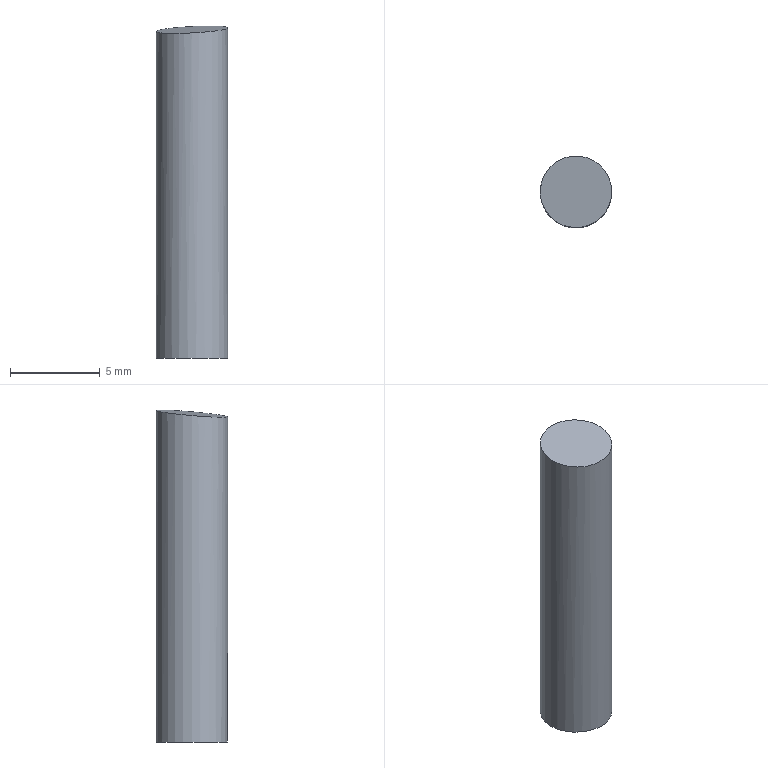Part | NX | features solid 2 | 1 solid | 3 faces | box 4 x 4 x 18.548 mm | volume 230.472 mm3 | plane 2 | cylinder 1 | commonest cylinder face diameters 4 x1
STEP:
#1=CARTESIAN_POINT('',(-212.753,0.1299,-24.));
#2=VERTEX_POINT('',#1);
#3=CARTESIAN_POINT('',(-210.753,0.1299,-24.));
#4=DIRECTION('',(0.,0.,-1.));
#5=DIRECTION('',(-1.,0.,0.));
#6=AXIS2_PLACEMENT_3D('',#3,#4,#5);
#7=CIRCLE('',#6,2.);
#8=EDGE_CURVE('',#2,#2,#7,.F.);
#9=ORIENTED_EDGE('',*,*,#8,.F.);
#10=EDGE_LOOP('',(#9));
#11=FACE_BOUND('',#10,.T.);
#12=CARTESIAN_POINT('',(-190.896,-11.477,-24.));
#13=DIRECTION('',(0.,0.,-1.));
#14=DIRECTION('',(-1.,0.,0.));
#15=AXIS2_PLACEMENT_3D('',#12,#13,#14);
#16=PLANE('',#15);
#17=ADVANCED_FACE('',(#11),#16,.T.);
#18=CARTESIAN_POINT('',(-211.762,-1.597,-5.867));
#19=VERTEX_POINT('',#18);
#20=CARTESIAN_POINT('',(-210.753,0.1299,-5.66));
#21=DIRECTION('',(0.05204,0.08903,-0.9947));
#22=DIRECTION('',(-0.502,-0.8587,-0.1031));
#23=AXIS2_PLACEMENT_3D('',#20,#21,#22);
#24=ELLIPSE('',#23,2.011,2.);
#25=EDGE_CURVE('',#19,#19,#24,.T.);
#26=ORIENTED_EDGE('',*,*,#25,.F.);
#27=EDGE_LOOP('',(#26));
#28=FACE_BOUND('',#27,.T.);
#29=CARTESIAN_POINT('',(-119.296,15.161,0.4708));
#30=DIRECTION('',(0.05204,0.08903,-0.9947));
#31=DIRECTION('',(0.005002,-0.996,-0.08889));
#32=AXIS2_PLACEMENT_3D('',#29,#30,#31);
#33=PLANE('',#32);
#34=ADVANCED_FACE('',(#28),#33,.F.);
#35=ORIENTED_EDGE('',*,*,#8,.T.);
#36=EDGE_LOOP('',(#35));
#37=FACE_BOUND('',#36,.T.);
#38=ORIENTED_EDGE('',*,*,#25,.T.);
#39=EDGE_LOOP('',(#38));
#40=FACE_BOUND('',#39,.T.);
#41=CARTESIAN_POINT('',(-210.753,0.1299,-2.666));
#42=DIRECTION('',(0.,0.,-1.));
#43=DIRECTION('',(-1.,0.,0.));
#44=AXIS2_PLACEMENT_3D('',#41,#42,#43);
#45=CYLINDRICAL_SURFACE('',#44,2.);
#46=ADVANCED_FACE('',(#37,#40),#45,.T.);
#47=CLOSED_SHELL('',(#17,#34,#46));
#48=MANIFOLD_SOLID_BREP('',#47);
#49=(LENGTH_UNIT()NAMED_UNIT(*)SI_UNIT(.MILLI.,.METRE.));
#50=UNCERTAINTY_MEASURE_WITH_UNIT(LENGTH_MEASURE(0.00001),#49,'','');
#51=(NAMED_UNIT(*)PLANE_ANGLE_UNIT()SI_UNIT($,.RADIAN.));
#52=(NAMED_UNIT(*)SI_UNIT($,.STERADIAN.)SOLID_ANGLE_UNIT());
#53=(GEOMETRIC_REPRESENTATION_CONTEXT(3)GLOBAL_UNCERTAINTY_ASSIGNED_CONTEXT((#50))GLOBAL_UNIT_ASSIGNED_CONTEXT((#49,#51,#52))REPRESENTATION_CONTEXT('',''));
#54=ADVANCED_BREP_SHAPE_REPRESENTATION('',(#48),#53);